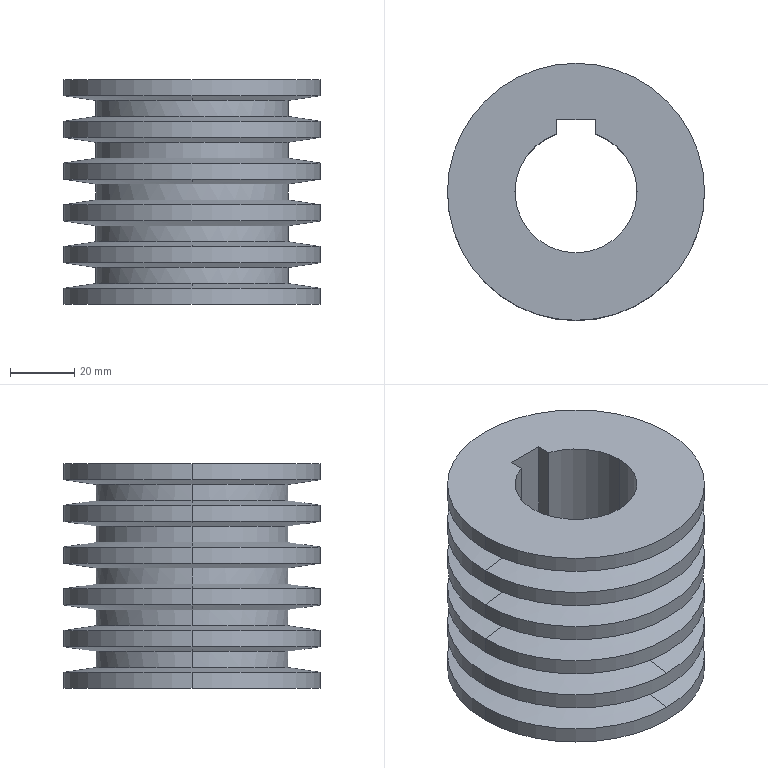Part | SolidWorks | 1 solid | 50 faces | box 80 x 80 x 70 mm | volume 197004 mm3 | cylinder 25 | cone 20 | plane 5 | commonest cylinder face diameters 80 x12 60 x10 38 x3
STEP:
#1=CARTESIAN_POINT('',(6.,18.028,-70.));
#2=VERTEX_POINT('',#1);
#3=CARTESIAN_POINT('',(6.,18.028,0.));
#4=VERTEX_POINT('',#3);
#5=CARTESIAN_POINT('',(6.,18.028,-70.));
#6=DIRECTION('',(0.,0.,1.));
#7=VECTOR('',#6,1000.);
#8=LINE('',#5,#7);
#9=EDGE_CURVE('',#2,#4,#8,.T.);
#10=ORIENTED_EDGE('',*,*,#9,.T.);
#11=CARTESIAN_POINT('',(6.,22.5,0.));
#12=VERTEX_POINT('',#11);
#13=CARTESIAN_POINT('',(6.,22.5,0.));
#14=DIRECTION('',(0.,-1.,0.));
#15=VECTOR('',#14,1000.);
#16=LINE('',#13,#15);
#17=EDGE_CURVE('',#12,#4,#16,.T.);
#18=ORIENTED_EDGE('',*,*,#17,.F.);
#19=CARTESIAN_POINT('',(6.,22.5,-70.));
#20=VERTEX_POINT('',#19);
#21=CARTESIAN_POINT('',(6.,22.5,0.));
#22=DIRECTION('',(0.,0.,-1.));
#23=VECTOR('',#22,1000.);
#24=LINE('',#21,#23);
#25=EDGE_CURVE('',#12,#20,#24,.T.);
#26=ORIENTED_EDGE('',*,*,#25,.T.);
#27=CARTESIAN_POINT('',(6.,18.028,-70.));
#28=DIRECTION('',(0.,1.,0.));
#29=VECTOR('',#28,1000.);
#30=LINE('',#27,#29);
#31=EDGE_CURVE('',#2,#20,#30,.T.);
#32=ORIENTED_EDGE('',*,*,#31,.F.);
#33=EDGE_LOOP('',(#10,#18,#26,#32));
#34=FACE_OUTER_BOUND('',#33,.T.);
#35=CARTESIAN_POINT('',(6.,22.5,-70.));
#36=DIRECTION('',(1.,0.,0.));
#37=DIRECTION('',(0.,1.,0.));
#38=AXIS2_PLACEMENT_3D('',#35,#36,#37);
#39=PLANE('',#38);
#40=ADVANCED_FACE('',(#34),#39,.F.);
#41=CARTESIAN_POINT('',(19.,0.,0.));
#42=VERTEX_POINT('',#41);
#43=CARTESIAN_POINT('',(0.,0.,0.));
#44=DIRECTION('',(0.,0.,1.));
#45=DIRECTION('',(1.,0.,0.));
#46=AXIS2_PLACEMENT_3D('',#43,#44,#45);
#47=CIRCLE('',#46,19.);
#48=EDGE_CURVE('',#42,#4,#47,.T.);
#49=ORIENTED_EDGE('',*,*,#48,.T.);
#50=ORIENTED_EDGE('',*,*,#9,.F.);
#51=CARTESIAN_POINT('',(19.,0.,-70.));
#52=VERTEX_POINT('',#51);
#53=CARTESIAN_POINT('',(0.,0.,-70.));
#54=DIRECTION('',(0.,0.,-1.));
#55=DIRECTION('',(0.3158,0.9488,0.));
#56=AXIS2_PLACEMENT_3D('',#53,#54,#55);
#57=CIRCLE('',#56,19.);
#58=EDGE_CURVE('',#2,#52,#57,.T.);
#59=ORIENTED_EDGE('',*,*,#58,.T.);
#60=CARTESIAN_POINT('',(19.,0.,-70.));
#61=DIRECTION('',(0.,0.,1.));
#62=VECTOR('',#61,1000.);
#63=LINE('',#60,#62);
#64=EDGE_CURVE('',#52,#42,#63,.T.);
#65=ORIENTED_EDGE('',*,*,#64,.T.);
#66=EDGE_LOOP('',(#49,#50,#59,#65));
#67=FACE_OUTER_BOUND('',#66,.T.);
#68=CARTESIAN_POINT('',(0.,0.,0.));
#69=DIRECTION('',(0.,0.,1.));
#70=DIRECTION('',(1.,0.,0.));
#71=AXIS2_PLACEMENT_3D('',#68,#69,#70);
#72=CYLINDRICAL_SURFACE('',#71,19.);
#73=ADVANCED_FACE('',(#67),#72,.F.);
#74=CARTESIAN_POINT('',(-6.,22.5,0.));
#75=VERTEX_POINT('',#74);
#76=CARTESIAN_POINT('',(-6.,22.5,-70.));
#77=VERTEX_POINT('',#76);
#78=CARTESIAN_POINT('',(-6.,22.5,0.));
#79=DIRECTION('',(0.,0.,-1.));
#80=VECTOR('',#79,1000.);
#81=LINE('',#78,#80);
#82=EDGE_CURVE('',#75,#77,#81,.T.);
#83=ORIENTED_EDGE('',*,*,#82,.F.);
#84=CARTESIAN_POINT('',(-6.,18.028,0.));
#85=VERTEX_POINT('',#84);
#86=CARTESIAN_POINT('',(-6.,18.028,0.));
#87=DIRECTION('',(0.,1.,0.));
#88=VECTOR('',#87,1000.);
#89=LINE('',#86,#88);
#90=EDGE_CURVE('',#85,#75,#89,.T.);
#91=ORIENTED_EDGE('',*,*,#90,.F.);
#92=CARTESIAN_POINT('',(-6.,18.028,-70.));
#93=VERTEX_POINT('',#92);
#94=CARTESIAN_POINT('',(-6.,18.028,0.));
#95=DIRECTION('',(0.,0.,-1.));
#96=VECTOR('',#95,1000.);
#97=LINE('',#94,#96);
#98=EDGE_CURVE('',#85,#93,#97,.T.);
#99=ORIENTED_EDGE('',*,*,#98,.T.);
#100=CARTESIAN_POINT('',(-6.,22.5,-70.));
#101=DIRECTION('',(0.,-1.,0.));
#102=VECTOR('',#101,1000.);
#103=LINE('',#100,#102);
#104=EDGE_CURVE('',#77,#93,#103,.T.);
#105=ORIENTED_EDGE('',*,*,#104,.F.);
#106=EDGE_LOOP('',(#83,#91,#99,#105));
#107=FACE_OUTER_BOUND('',#106,.T.);
#108=CARTESIAN_POINT('',(-6.,22.5,-70.));
#109=DIRECTION('',(-1.,0.,0.));
#110=DIRECTION('',(0.,0.,1.));
#111=AXIS2_PLACEMENT_3D('',#108,#109,#110);
#112=PLANE('',#111);
#113=ADVANCED_FACE('',(#107),#112,.F.);
#114=ORIENTED_EDGE('',*,*,#98,.F.);
#115=CARTESIAN_POINT('',(-19.,0.,0.));
#116=VERTEX_POINT('',#115);
#117=CARTESIAN_POINT('',(0.,0.,0.));
#118=DIRECTION('',(0.,0.,1.));
#119=DIRECTION('',(-0.3158,0.9488,0.));
#120=AXIS2_PLACEMENT_3D('',#117,#118,#119);
#121=CIRCLE('',#120,19.);
#122=EDGE_CURVE('',#85,#116,#121,.T.);
#123=ORIENTED_EDGE('',*,*,#122,.T.);
#124=CARTESIAN_POINT('',(-19.,0.,-70.));
#125=VERTEX_POINT('',#124);
#126=CARTESIAN_POINT('',(-19.,0.,-70.));
#127=DIRECTION('',(0.,0.,1.));
#128=VECTOR('',#127,1000.);
#129=LINE('',#126,#128);
#130=EDGE_CURVE('',#125,#116,#129,.T.);
#131=ORIENTED_EDGE('',*,*,#130,.F.);
#132=CARTESIAN_POINT('',(0.,0.,-70.));
#133=DIRECTION('',(0.,0.,-1.));
#134=DIRECTION('',(-1.,0.,0.));
#135=AXIS2_PLACEMENT_3D('',#132,#133,#134);
#136=CIRCLE('',#135,19.);
#137=EDGE_CURVE('',#125,#93,#136,.T.);
#138=ORIENTED_EDGE('',*,*,#137,.T.);
#139=EDGE_LOOP('',(#114,#123,#131,#138));
#140=FACE_OUTER_BOUND('',#139,.T.);
#141=CARTESIAN_POINT('',(0.,0.,0.));
#142=DIRECTION('',(0.,0.,1.));
#143=DIRECTION('',(1.,0.,0.));
#144=AXIS2_PLACEMENT_3D('',#141,#142,#143);
#145=CYLINDRICAL_SURFACE('',#144,19.);
#146=ADVANCED_FACE('',(#140),#145,.F.);
#147=CARTESIAN_POINT('',(0.,0.,0.));
#148=DIRECTION('',(0.,0.,1.));
#149=DIRECTION('',(-1.,0.,0.));
#150=AXIS2_PLACEMENT_3D('',#147,#148,#149);
#151=CIRCLE('',#150,19.);
#152=EDGE_CURVE('',#116,#42,#151,.T.);
#153=ORIENTED_EDGE('',*,*,#152,.T.);
#154=ORIENTED_EDGE('',*,*,#64,.F.);
#155=CARTESIAN_POINT('',(0.,0.,-70.));
#156=DIRECTION('',(0.,0.,-1.));
#157=DIRECTION('',(1.,0.,0.));
#158=AXIS2_PLACEMENT_3D('',#155,#156,#157);
#159=CIRCLE('',#158,19.);
#160=EDGE_CURVE('',#52,#125,#159,.T.);
#161=ORIENTED_EDGE('',*,*,#160,.T.);
#162=ORIENTED_EDGE('',*,*,#130,.T.);
#163=EDGE_LOOP('',(#153,#154,#161,#162));
#164=FACE_OUTER_BOUND('',#163,.T.);
#165=CARTESIAN_POINT('',(0.,0.,0.));
#166=DIRECTION('',(0.,0.,1.));
#167=DIRECTION('',(1.,0.,0.));
#168=AXIS2_PLACEMENT_3D('',#165,#166,#167);
#169=CYLINDRICAL_SURFACE('',#168,19.);
#170=ADVANCED_FACE('',(#164),#169,.F.);
#171=CARTESIAN_POINT('',(-40.,0.,-52.));
#172=VERTEX_POINT('',#171);
#173=CARTESIAN_POINT('',(0.,40.,-52.));
#174=VERTEX_POINT('',#173);
#175=CARTESIAN_POINT('',(0.,0.,-52.));
#176=DIRECTION('',(0.,0.,-1.));
#177=DIRECTION('',(-1.,0.,0.));
#178=AXIS2_PLACEMENT_3D('',#175,#176,#177);
#179=CIRCLE('',#178,40.);
#180=EDGE_CURVE('',#172,#174,#179,.T.);
#181=ORIENTED_EDGE('',*,*,#180,.T.);
#182=CARTESIAN_POINT('',(40.,0.,-52.));
#183=VERTEX_POINT('',#182);
#184=CARTESIAN_POINT('',(0.,0.,-52.));
#185=DIRECTION('',(0.,0.,-1.));
#186=DIRECTION('',(0.,1.,0.));
#187=AXIS2_PLACEMENT_3D('',#184,#185,#186);
#188=CIRCLE('',#187,40.);
#189=EDGE_CURVE('',#174,#183,#188,.T.);
#190=ORIENTED_EDGE('',*,*,#189,.T.);
#191=CARTESIAN_POINT('',(40.,0.,-57.));
#192=VERTEX_POINT('',#191);
#193=CARTESIAN_POINT('',(40.,0.,-57.));
#194=DIRECTION('',(0.,0.,1.));
#195=VECTOR('',#194,1000.);
#196=LINE('',#193,#195);
#197=EDGE_CURVE('',#192,#183,#196,.T.);
#198=ORIENTED_EDGE('',*,*,#197,.F.);
#199=CARTESIAN_POINT('',(-40.,0.,-57.));
#200=VERTEX_POINT('',#199);
#201=CARTESIAN_POINT('',(0.,0.,-57.));
#202=DIRECTION('',(0.,0.,1.));
#203=DIRECTION('',(1.,0.,0.));
#204=AXIS2_PLACEMENT_3D('',#201,#202,#203);
#205=CIRCLE('',#204,40.);
#206=EDGE_CURVE('',#192,#200,#205,.T.);
#207=ORIENTED_EDGE('',*,*,#206,.T.);
#208=CARTESIAN_POINT('',(-40.,0.,-57.));
#209=DIRECTION('',(0.,0.,1.));
#210=VECTOR('',#209,1000.);
#211=LINE('',#208,#210);
#212=EDGE_CURVE('',#200,#172,#211,.T.);
#213=ORIENTED_EDGE('',*,*,#212,.T.);
#214=EDGE_LOOP('',(#181,#190,#198,#207,#213));
#215=FACE_OUTER_BOUND('',#214,.T.);
#216=CARTESIAN_POINT('',(0.,0.,0.));
#217=DIRECTION('',(0.,0.,1.));
#218=DIRECTION('',(1.,0.,0.));
#219=AXIS2_PLACEMENT_3D('',#216,#217,#218);
#220=CYLINDRICAL_SURFACE('',#219,40.);
#221=ADVANCED_FACE('',(#215),#220,.T.);
#222=ORIENTED_EDGE('',*,*,#197,.T.);
#223=CARTESIAN_POINT('',(0.,-40.,-52.));
#224=VERTEX_POINT('',#223);
#225=CARTESIAN_POINT('',(0.,0.,-52.));
#226=DIRECTION('',(0.,0.,-1.));
#227=DIRECTION('',(1.,0.,0.));
#228=AXIS2_PLACEMENT_3D('',#225,#226,#227);
#229=CIRCLE('',#228,40.);
#230=EDGE_CURVE('',#183,#224,#229,.T.);
#231=ORIENTED_EDGE('',*,*,#230,.T.);
#232=CARTESIAN_POINT('',(0.,0.,-52.));
#233=DIRECTION('',(0.,0.,-1.));
#234=DIRECTION('',(0.,-1.,0.));
#235=AXIS2_PLACEMENT_3D('',#232,#233,#234);
#236=CIRCLE('',#235,40.);
#237=EDGE_CURVE('',#224,#172,#236,.T.);
#238=ORIENTED_EDGE('',*,*,#237,.T.);
#239=ORIENTED_EDGE('',*,*,#212,.F.);
#240=CARTESIAN_POINT('',(0.,0.,-57.));
#241=DIRECTION('',(0.,0.,1.));
#242=DIRECTION('',(-1.,0.,0.));
#243=AXIS2_PLACEMENT_3D('',#240,#241,#242);
#244=CIRCLE('',#243,40.);
#245=EDGE_CURVE('',#200,#192,#244,.T.);
#246=ORIENTED_EDGE('',*,*,#245,.T.);
#247=EDGE_LOOP('',(#222,#231,#238,#239,#246));
#248=FACE_OUTER_BOUND('',#247,.T.);
#249=CARTESIAN_POINT('',(0.,0.,0.));
#250=DIRECTION('',(0.,0.,1.));
#251=DIRECTION('',(1.,0.,0.));
#252=AXIS2_PLACEMENT_3D('',#249,#250,#251);
#253=CYLINDRICAL_SURFACE('',#252,40.);
#254=ADVANCED_FACE('',(#248),#253,.T.);
#255=CARTESIAN_POINT('',(30.,0.,-58.5));
#256=VERTEX_POINT('',#255);
#257=CARTESIAN_POINT('',(30.,0.,-58.5));
#258=DIRECTION('',(0.9889,0.,0.1483));
#259=VECTOR('',#258,1000.);
#260=LINE('',#257,#259);
#261=EDGE_CURVE('',#256,#192,#260,.T.);
#262=ORIENTED_EDGE('',*,*,#261,.T.);
#263=ORIENTED_EDGE('',*,*,#245,.F.);
#264=CARTESIAN_POINT('',(-30.,0.,-58.5));
#265=VERTEX_POINT('',#264);
#266=CARTESIAN_POINT('',(-30.,0.,-58.5));
#267=DIRECTION('',(-0.9889,0.,0.1483));
#268=VECTOR('',#267,1000.);
#269=LINE('',#266,#268);
#270=EDGE_CURVE('',#265,#200,#269,.T.);
#271=ORIENTED_EDGE('',*,*,#270,.F.);
#272=CARTESIAN_POINT('',(0.,0.,-58.5));
#273=DIRECTION('',(0.,0.,-1.));
#274=DIRECTION('',(1.,0.,0.));
#275=AXIS2_PLACEMENT_3D('',#272,#273,#274);
#276=CIRCLE('',#275,30.);
#277=EDGE_CURVE('',#256,#265,#276,.T.);
#278=ORIENTED_EDGE('',*,*,#277,.F.);
#279=EDGE_LOOP('',(#262,#263,#271,#278));
#280=FACE_OUTER_BOUND('',#279,.T.);
#281=CARTESIAN_POINT('',(0.,0.,-58.53));
#282=DIRECTION('',(0.,0.,1.));
#283=DIRECTION('',(1.,0.,0.));
#284=AXIS2_PLACEMENT_3D('',#281,#282,#283);
#285=CONICAL_SURFACE('',#284,29.8,1.422);
#286=ADVANCED_FACE('',(#280),#285,.T.);
#287=ORIENTED_EDGE('',*,*,#206,.F.);
#288=ORIENTED_EDGE('',*,*,#261,.F.);
#289=CARTESIAN_POINT('',(0.,0.,-58.5));
#290=DIRECTION('',(0.,0.,-1.));
#291=DIRECTION('',(-1.,0.,0.));
#292=AXIS2_PLACEMENT_3D('',#289,#290,#291);
#293=CIRCLE('',#292,30.);
#294=EDGE_CURVE('',#265,#256,#293,.T.);
#295=ORIENTED_EDGE('',*,*,#294,.F.);
#296=ORIENTED_EDGE('',*,*,#270,.T.);
#297=EDGE_LOOP('',(#287,#288,#295,#296));
#298=FACE_OUTER_BOUND('',#297,.T.);
#299=CARTESIAN_POINT('',(0.,0.,-58.53));
#300=DIRECTION('',(0.,0.,1.));
#301=DIRECTION('',(1.,0.,0.));
#302=AXIS2_PLACEMENT_3D('',#299,#300,#301);
#303=CONICAL_SURFACE('',#302,29.8,1.422);
#304=ADVANCED_FACE('',(#298),#303,.T.);
#305=CARTESIAN_POINT('',(40.,0.,-65.));
#306=VERTEX_POINT('',#305);
#307=CARTESIAN_POINT('',(0.,-40.,-65.));
#308=VERTEX_POINT('',#307);
#309=CARTESIAN_POINT('',(0.,0.,-65.));
#310=DIRECTION('',(0.,0.,-1.));
#311=DIRECTION('',(1.,0.,0.));
#312=AXIS2_PLACEMENT_3D('',#309,#310,#311);
#313=CIRCLE('',#312,40.);
#314=EDGE_CURVE('',#306,#308,#313,.T.);
#315=ORIENTED_EDGE('',*,*,#314,.F.);
#316=CARTESIAN_POINT('',(0.,40.,-65.));
#317=VERTEX_POINT('',#316);
#318=CARTESIAN_POINT('',(0.,0.,-65.));
#319=DIRECTION('',(0.,0.,-1.));
#320=DIRECTION('',(0.,1.,0.));
#321=AXIS2_PLACEMENT_3D('',#318,#319,#320);
#322=CIRCLE('',#321,40.);
#323=EDGE_CURVE('',#317,#306,#322,.T.);
#324=ORIENTED_EDGE('',*,*,#323,.F.);
#325=CARTESIAN_POINT('',(0.,30.,-63.5));
#326=VERTEX_POINT('',#325);
#327=CARTESIAN_POINT('',(0.,30.,-63.5));
#328=DIRECTION('',(0.,0.9889,-0.1483));
#329=VECTOR('',#328,1000.);
#330=LINE('',#327,#329);
#331=EDGE_CURVE('',#326,#317,#330,.T.);
#332=ORIENTED_EDGE('',*,*,#331,.F.);
#333=CARTESIAN_POINT('',(30.,0.,-63.5));
#334=VERTEX_POINT('',#333);
#335=CARTESIAN_POINT('',(0.,0.,-63.5));
#336=DIRECTION('',(0.,0.,1.));
#337=DIRECTION('',(1.,0.,0.));
#338=AXIS2_PLACEMENT_3D('',#335,#336,#337);
#339=CIRCLE('',#338,30.);
#340=EDGE_CURVE('',#334,#326,#339,.T.);
#341=ORIENTED_EDGE('',*,*,#340,.F.);
#342=CARTESIAN_POINT('',(0.,-30.,-63.5));
#343=VERTEX_POINT('',#342);
#344=CARTESIAN_POINT('',(0.,0.,-63.5));
#345=DIRECTION('',(0.,0.,1.));
#346=DIRECTION('',(0.,-1.,0.));
#347=AXIS2_PLACEMENT_3D('',#344,#345,#346);
#348=CIRCLE('',#347,30.);
#349=EDGE_CURVE('',#343,#334,#348,.T.);
#350=ORIENTED_EDGE('',*,*,#349,.F.);
#351=CARTESIAN_POINT('',(0.,-30.,-63.5));
#352=DIRECTION('',(0.,-0.9889,-0.1483));
#353=VECTOR('',#352,1000.);
#354=LINE('',#351,#353);
#355=EDGE_CURVE('',#343,#308,#354,.T.);
#356=ORIENTED_EDGE('',*,*,#355,.T.);
#357=EDGE_LOOP('',(#315,#324,#332,#341,#350,#356));
#358=FACE_OUTER_BOUND('',#357,.T.);
#359=CARTESIAN_POINT('',(0.,0.,-63.47));
#360=DIRECTION('',(0.,0.,-1.));
#361=DIRECTION('',(0.,1.,0.));
#362=AXIS2_PLACEMENT_3D('',#359,#360,#361);
#363=CONICAL_SURFACE('',#362,29.8,1.422);
#364=ADVANCED_FACE('',(#358),#363,.T.);
#365=ORIENTED_EDGE('',*,*,#294,.T.);
#366=CARTESIAN_POINT('',(30.,0.,-63.5));
#367=DIRECTION('',(0.,0.,1.));
#368=VECTOR('',#367,1000.);
#369=LINE('',#366,#368);
#370=EDGE_CURVE('',#334,#256,#369,.T.);
#371=ORIENTED_EDGE('',*,*,#370,.F.);
#372=ORIENTED_EDGE('',*,*,#340,.T.);
#373=CARTESIAN_POINT('',(-30.,0.,-63.5));
#374=VERTEX_POINT('',#373);
#375=CARTESIAN_POINT('',(0.,0.,-63.5));
#376=DIRECTION('',(0.,0.,1.));
#377=DIRECTION('',(0.,1.,0.));
#378=AXIS2_PLACEMENT_3D('',#375,#376,#377);
#379=CIRCLE('',#378,30.);
#380=EDGE_CURVE('',#326,#374,#379,.T.);
#381=ORIENTED_EDGE('',*,*,#380,.T.);
#382=CARTESIAN_POINT('',(-30.,0.,-63.5));
#383=DIRECTION('',(0.,0.,1.));
#384=VECTOR('',#383,1000.);
#385=LINE('',#382,#384);
#386=EDGE_CURVE('',#374,#265,#385,.T.);
#387=ORIENTED_EDGE('',*,*,#386,.T.);
#388=EDGE_LOOP('',(#365,#371,#372,#381,#387));
#389=FACE_OUTER_BOUND('',#388,.T.);
#390=CARTESIAN_POINT('',(0.,0.,0.));
#391=DIRECTION('',(0.,0.,1.));
#392=DIRECTION('',(1.,0.,0.));
#393=AXIS2_PLACEMENT_3D('',#390,#391,#392);
#394=CYLINDRICAL_SURFACE('',#393,30.);
#395=ADVANCED_FACE('',(#389),#394,.T.);
#396=ORIENTED_EDGE('',*,*,#349,.T.);
#397=ORIENTED_EDGE('',*,*,#370,.T.);
#398=ORIENTED_EDGE('',*,*,#277,.T.);
#399=ORIENTED_EDGE('',*,*,#386,.F.);
#400=CARTESIAN_POINT('',(0.,0.,-63.5));
#401=DIRECTION('',(0.,0.,1.));
#402=DIRECTION('',(-1.,0.,0.));
#403=AXIS2_PLACEMENT_3D('',#400,#401,#402);
#404=CIRCLE('',#403,30.);
#405=EDGE_CURVE('',#374,#343,#404,.T.);
#406=ORIENTED_EDGE('',*,*,#405,.T.);
#407=EDGE_LOOP('',(#396,#397,#398,#399,#406));
#408=FACE_OUTER_BOUND('',#407,.T.);
#409=CARTESIAN_POINT('',(0.,0.,0.));
#410=DIRECTION('',(0.,0.,1.));
#411=DIRECTION('',(1.,0.,0.));
#412=AXIS2_PLACEMENT_3D('',#409,#410,#411);
#413=CYLINDRICAL_SURFACE('',#412,30.);
#414=ADVANCED_FACE('',(#408),#413,.T.);
#415=ORIENTED_EDGE('',*,*,#380,.F.);
#416=ORIENTED_EDGE('',*,*,#331,.T.);
#417=CARTESIAN_POINT('',(-40.,0.,-65.));
#418=VERTEX_POINT('',#417);
#419=CARTESIAN_POINT('',(0.,0.,-65.));
#420=DIRECTION('',(0.,0.,-1.));
#421=DIRECTION('',(-1.,0.,0.));
#422=AXIS2_PLACEMENT_3D('',#419,#420,#421);
#423=CIRCLE('',#422,40.);
#424=EDGE_CURVE('',#418,#317,#423,.T.);
#425=ORIENTED_EDGE('',*,*,#424,.F.);
#426=CARTESIAN_POINT('',(0.,0.,-65.));
#427=DIRECTION('',(0.,0.,-1.));
#428=DIRECTION('',(0.,-1.,0.));
#429=AXIS2_PLACEMENT_3D('',#426,#427,#428);
#430=CIRCLE('',#429,40.);
#431=EDGE_CURVE('',#308,#418,#430,.T.);
#432=ORIENTED_EDGE('',*,*,#431,.F.);
#433=ORIENTED_EDGE('',*,*,#355,.F.);
#434=ORIENTED_EDGE('',*,*,#405,.F.);
#435=EDGE_LOOP('',(#415,#416,#425,#432,#433,#434));
#436=FACE_OUTER_BOUND('',#435,.T.);
#437=CARTESIAN_POINT('',(0.,0.,-63.47));
#438=DIRECTION('',(0.,0.,-1.));
#439=DIRECTION('',(0.,1.,0.));
#440=AXIS2_PLACEMENT_3D('',#437,#438,#439);
#441=CONICAL_SURFACE('',#440,29.8,1.422);
#442=ADVANCED_FACE('',(#436),#441,.T.);
#443=CARTESIAN_POINT('',(40.,0.,-70.));
#444=VERTEX_POINT('',#443);
#445=CARTESIAN_POINT('',(40.,0.,-70.));
#446=DIRECTION('',(0.,0.,1.));
#447=VECTOR('',#446,1000.);
#448=LINE('',#445,#447);
#449=EDGE_CURVE('',#444,#306,#448,.T.);
#450=ORIENTED_EDGE('',*,*,#449,.T.);
#451=ORIENTED_EDGE('',*,*,#314,.T.);
#452=ORIENTED_EDGE('',*,*,#431,.T.);
#453=CARTESIAN_POINT('',(-40.,0.,-70.));
#454=VERTEX_POINT('',#453);
#455=CARTESIAN_POINT('',(-40.,0.,-70.));
#456=DIRECTION('',(0.,0.,1.));
#457=VECTOR('',#456,1000.);
#458=LINE('',#455,#457);
#459=EDGE_CURVE('',#454,#418,#458,.T.);
#460=ORIENTED_EDGE('',*,*,#459,.F.);
#461=CARTESIAN_POINT('',(0.,0.,-70.));
#462=DIRECTION('',(0.,0.,1.));
#463=DIRECTION('',(-1.,0.,0.));
#464=AXIS2_PLACEMENT_3D('',#461,#462,#463);
#465=CIRCLE('',#464,40.);
#466=EDGE_CURVE('',#454,#444,#465,.T.);
#467=ORIENTED_EDGE('',*,*,#466,.T.);
#468=EDGE_LOOP('',(#450,#451,#452,#460,#467));
#469=FACE_OUTER_BOUND('',#468,.T.);
#470=CARTESIAN_POINT('',(0.,0.,0.));
#471=DIRECTION('',(0.,0.,1.));
#472=DIRECTION('',(1.,0.,0.));
#473=AXIS2_PLACEMENT_3D('',#470,#471,#472);
#474=CYLINDRICAL_SURFACE('',#473,40.);
#475=ADVANCED_FACE('',(#469),#474,.T.);
#476=ORIENTED_EDGE('',*,*,#424,.T.);
#477=ORIENTED_EDGE('',*,*,#323,.T.);
#478=ORIENTED_EDGE('',*,*,#449,.F.);
#479=CARTESIAN_POINT('',(0.,0.,-70.));
#480=DIRECTION('',(0.,0.,1.));
#481=DIRECTION('',(1.,0.,0.));
#482=AXIS2_PLACEMENT_3D('',#479,#480,#481);
#483=CIRCLE('',#482,40.);
#484=EDGE_CURVE('',#444,#454,#483,.T.);
#485=ORIENTED_EDGE('',*,*,#484,.T.);
#486=ORIENTED_EDGE('',*,*,#459,.T.);
#487=EDGE_LOOP('',(#476,#477,#478,#485,#486));
#488=FACE_OUTER_BOUND('',#487,.T.);
#489=CARTESIAN_POINT('',(0.,0.,0.));
#490=DIRECTION('',(0.,0.,1.));
#491=DIRECTION('',(1.,0.,0.));
#492=AXIS2_PLACEMENT_3D('',#489,#490,#491);
#493=CYLINDRICAL_SURFACE('',#492,40.);
#494=ADVANCED_FACE('',(#488),#493,.T.);
#495=ORIENTED_EDGE('',*,*,#58,.F.);
#496=ORIENTED_EDGE('',*,*,#31,.T.);
#497=CARTESIAN_POINT('',(6.,22.5,-70.));
#498=DIRECTION('',(-1.,0.,0.));
#499=VECTOR('',#498,1000.);
#500=LINE('',#497,#499);
#501=EDGE_CURVE('',#20,#77,#500,.T.);
#502=ORIENTED_EDGE('',*,*,#501,.T.);
#503=ORIENTED_EDGE('',*,*,#104,.T.);
#504=ORIENTED_EDGE('',*,*,#137,.F.);
#505=ORIENTED_EDGE('',*,*,#160,.F.);
#506=EDGE_LOOP('',(#495,#496,#502,#503,#504,#505));
#507=FACE_BOUND('',#506,.T.);
#508=ORIENTED_EDGE('',*,*,#466,.F.);
#509=ORIENTED_EDGE('',*,*,#484,.F.);
#510=EDGE_LOOP('',(#508,#509));
#511=FACE_OUTER_BOUND('',#510,.T.);
#512=CARTESIAN_POINT('',(0.,-40.,-70.));
#513=DIRECTION('',(0.,0.,-1.));
#514=DIRECTION('',(0.,-1.,0.));
#515=AXIS2_PLACEMENT_3D('',#512,#513,#514);
#516=PLANE('',#515);
#517=ADVANCED_FACE('',(#507,#511),#516,.T.);
#518=ORIENTED_EDGE('',*,*,#25,.F.);
#519=CARTESIAN_POINT('',(-6.,22.5,0.));
#520=DIRECTION('',(1.,0.,0.));
#521=VECTOR('',#520,1000.);
#522=LINE('',#519,#521);
#523=EDGE_CURVE('',#75,#12,#522,.T.);
#524=ORIENTED_EDGE('',*,*,#523,.F.);
#525=ORIENTED_EDGE('',*,*,#82,.T.);
#526=ORIENTED_EDGE('',*,*,#501,.F.);
#527=EDGE_LOOP('',(#518,#524,#525,#526));
#528=FACE_OUTER_BOUND('',#527,.T.);
#529=CARTESIAN_POINT('',(0.,22.5,-70.));
#530=DIRECTION('',(0.,1.,0.));
#531=DIRECTION('',(1.,0.,0.));
#532=AXIS2_PLACEMENT_3D('',#529,#530,#531);
#533=PLANE('',#532);
#534=ADVANCED_FACE('',(#528),#533,.F.);
#535=ORIENTED_EDGE('',*,*,#17,.T.);
#536=ORIENTED_EDGE('',*,*,#48,.F.);
#537=ORIENTED_EDGE('',*,*,#152,.F.);
#538=ORIENTED_EDGE('',*,*,#122,.F.);
#539=ORIENTED_EDGE('',*,*,#90,.T.);
#540=ORIENTED_EDGE('',*,*,#523,.T.);
#541=EDGE_LOOP('',(#535,#536,#537,#538,#539,#540));
#542=FACE_BOUND('',#541,.T.);
#543=CARTESIAN_POINT('',(-40.,0.,0.));
#544=VERTEX_POINT('',#543);
#545=CARTESIAN_POINT('',(40.,0.,0.));
#546=VERTEX_POINT('',#545);
#547=CARTESIAN_POINT('',(0.,0.,0.));
#548=DIRECTION('',(0.,0.,-1.));
#549=DIRECTION('',(-1.,0.,0.));
#550=AXIS2_PLACEMENT_3D('',#547,#548,#549);
#551=CIRCLE('',#550,40.);
#552=EDGE_CURVE('',#544,#546,#551,.T.);
#553=ORIENTED_EDGE('',*,*,#552,.F.);
#554=CARTESIAN_POINT('',(0.,0.,0.));
#555=DIRECTION('',(0.,0.,-1.));
#556=DIRECTION('',(1.,0.,0.));
#557=AXIS2_PLACEMENT_3D('',#554,#555,#556);
#558=CIRCLE('',#557,40.);
#559=EDGE_CURVE('',#546,#544,#558,.T.);
#560=ORIENTED_EDGE('',*,*,#559,.F.);
#561=EDGE_LOOP('',(#553,#560));
#562=FACE_OUTER_BOUND('',#561,.T.);
#563=CARTESIAN_POINT('',(0.,-19.,0.));
#564=DIRECTION('',(0.,0.,1.));
#565=DIRECTION('',(1.,0.,0.));
#566=AXIS2_PLACEMENT_3D('',#563,#564,#565);
#567=PLANE('',#566);
#568=ADVANCED_FACE('',(#542,#562),#567,.T.);
#569=CARTESIAN_POINT('',(0.,-40.,-5.));
#570=VERTEX_POINT('',#569);
#571=CARTESIAN_POINT('',(40.,0.,-5.));
#572=VERTEX_POINT('',#571);
#573=CARTESIAN_POINT('',(0.,0.,-5.));
#574=DIRECTION('',(0.,0.,1.));
#575=DIRECTION('',(0.,-1.,0.));
#576=AXIS2_PLACEMENT_3D('',#573,#574,#575);
#577=CIRCLE('',#576,40.);
#578=EDGE_CURVE('',#570,#572,#577,.T.);
#579=ORIENTED_EDGE('',*,*,#578,.T.);
#580=CARTESIAN_POINT('',(40.,0.,-5.));
#581=DIRECTION('',(0.,0.,1.));
#582=VECTOR('',#581,1000.);
#583=LINE('',#580,#582);
#584=EDGE_CURVE('',#572,#546,#583,.T.);
#585=ORIENTED_EDGE('',*,*,#584,.T.);
#586=ORIENTED_EDGE('',*,*,#559,.T.);
#587=CARTESIAN_POINT('',(-40.,0.,-5.));
#588=VERTEX_POINT('',#587);
#589=CARTESIAN_POINT('',(-40.,0.,-5.));
#590=DIRECTION('',(0.,0.,1.));
#591=VECTOR('',#590,1000.);
#592=LINE('',#589,#591);
#593=EDGE_CURVE('',#588,#544,#592,.T.);
#594=ORIENTED_EDGE('',*,*,#593,.F.);
#595=CARTESIAN_POINT('',(0.,0.,-5.));
#596=DIRECTION('',(0.,0.,1.));
#597=DIRECTION('',(-1.,0.,0.));
#598=AXIS2_PLACEMENT_3D('',#595,#596,#597);
#599=CIRCLE('',#598,40.);
#600=EDGE_CURVE('',#588,#570,#599,.T.);
#601=ORIENTED_EDGE('',*,*,#600,.T.);
#602=EDGE_LOOP('',(#579,#585,#586,#594,#601));
#603=FACE_OUTER_BOUND('',#602,.T.);
#604=CARTESIAN_POINT('',(0.,0.,0.));
#605=DIRECTION('',(0.,0.,1.));
#606=DIRECTION('',(1.,0.,0.));
#607=AXIS2_PLACEMENT_3D('',#604,#605,#606);
#608=CYLINDRICAL_SURFACE('',#607,40.);
#609=ADVANCED_FACE('',(#603),#608,.T.);
#610=ORIENTED_EDGE('',*,*,#552,.T.);
#611=ORIENTED_EDGE('',*,*,#584,.F.);
#612=CARTESIAN_POINT('',(0.,40.,-5.));
#613=VERTEX_POINT('',#612);
#614=CARTESIAN_POINT('',(0.,0.,-5.));
#615=DIRECTION('',(0.,0.,1.));
#616=DIRECTION('',(1.,0.,0.));
#617=AXIS2_PLACEMENT_3D('',#614,#615,#616);
#618=CIRCLE('',#617,40.);
#619=EDGE_CURVE('',#572,#613,#618,.T.);
#620=ORIENTED_EDGE('',*,*,#619,.T.);
#621=CARTESIAN_POINT('',(0.,0.,-5.));
#622=DIRECTION('',(0.,0.,1.));
#623=DIRECTION('',(0.,1.,0.));
#624=AXIS2_PLACEMENT_3D('',#621,#622,#623);
#625=CIRCLE('',#624,40.);
#626=EDGE_CURVE('',#613,#588,#625,.T.);
#627=ORIENTED_EDGE('',*,*,#626,.T.);
#628=ORIENTED_EDGE('',*,*,#593,.T.);
#629=EDGE_LOOP('',(#610,#611,#620,#627,#628));
#630=FACE_OUTER_BOUND('',#629,.T.);
#631=CARTESIAN_POINT('',(0.,0.,0.));
#632=DIRECTION('',(0.,0.,1.));
#633=DIRECTION('',(1.,0.,0.));
#634=AXIS2_PLACEMENT_3D('',#631,#632,#633);
#635=CYLINDRICAL_SURFACE('',#634,40.);
#636=ADVANCED_FACE('',(#630),#635,.T.);
#637=CARTESIAN_POINT('',(0.,-30.,-6.5));
#638=VERTEX_POINT('',#637);
#639=CARTESIAN_POINT('',(-30.,0.,-6.5));
#640=VERTEX_POINT('',#639);
#641=CARTESIAN_POINT('',(0.,0.,-6.5));
#642=DIRECTION('',(0.,0.,-1.));
#643=DIRECTION('',(0.,-1.,0.));
#644=AXIS2_PLACEMENT_3D('',#641,#642,#643);
#645=CIRCLE('',#644,30.);
#646=EDGE_CURVE('',#638,#640,#645,.T.);
#647=ORIENTED_EDGE('',*,*,#646,.F.);
#648=CARTESIAN_POINT('',(0.,-30.,-6.5));
#649=DIRECTION('',(0.,-0.9889,0.1483));
#650=VECTOR('',#649,1000.);
#651=LINE('',#648,#650);
#652=EDGE_CURVE('',#638,#570,#651,.T.);
#653=ORIENTED_EDGE('',*,*,#652,.T.);
#654=ORIENTED_EDGE('',*,*,#600,.F.);
#655=ORIENTED_EDGE('',*,*,#626,.F.);
#656=CARTESIAN_POINT('',(0.,30.,-6.5));
#657=VERTEX_POINT('',#656);
#658=CARTESIAN_POINT('',(0.,30.,-6.5));
#659=DIRECTION('',(0.,0.9889,0.1483));
#660=VECTOR('',#659,1000.);
#661=LINE('',#658,#660);
#662=EDGE_CURVE('',#657,#613,#661,.T.);
#663=ORIENTED_EDGE('',*,*,#662,.F.);
#664=CARTESIAN_POINT('',(0.,0.,-6.5));
#665=DIRECTION('',(0.,0.,-1.));
#666=DIRECTION('',(-1.,0.,0.));
#667=AXIS2_PLACEMENT_3D('',#664,#665,#666);
#668=CIRCLE('',#667,30.);
#669=EDGE_CURVE('',#640,#657,#668,.T.);
#670=ORIENTED_EDGE('',*,*,#669,.F.);
#671=EDGE_LOOP('',(#647,#653,#654,#655,#663,#670));
#672=FACE_OUTER_BOUND('',#671,.T.);
#673=CARTESIAN_POINT('',(0.,0.,-6.53));
#674=DIRECTION('',(0.,0.,1.));
#675=DIRECTION('',(0.,-1.,0.));
#676=AXIS2_PLACEMENT_3D('',#673,#674,#675);
#677=CONICAL_SURFACE('',#676,29.8,1.422);
#678=ADVANCED_FACE('',(#672),#677,.T.);
#679=ORIENTED_EDGE('',*,*,#619,.F.);
#680=ORIENTED_EDGE('',*,*,#578,.F.);
#681=ORIENTED_EDGE('',*,*,#652,.F.);
#682=CARTESIAN_POINT('',(30.,0.,-6.5));
#683=VERTEX_POINT('',#682);
#684=CARTESIAN_POINT('',(0.,0.,-6.5));
#685=DIRECTION('',(0.,0.,-1.));
#686=DIRECTION('',(1.,0.,0.));
#687=AXIS2_PLACEMENT_3D('',#684,#685,#686);
#688=CIRCLE('',#687,30.);
#689=EDGE_CURVE('',#683,#638,#688,.T.);
#690=ORIENTED_EDGE('',*,*,#689,.F.);
#691=CARTESIAN_POINT('',(0.,0.,-6.5));
#692=DIRECTION('',(0.,0.,-1.));
#693=DIRECTION('',(0.,1.,0.));
#694=AXIS2_PLACEMENT_3D('',#691,#692,#693);
#695=CIRCLE('',#694,30.);
#696=EDGE_CURVE('',#657,#683,#695,.T.);
#697=ORIENTED_EDGE('',*,*,#696,.F.);
#698=ORIENTED_EDGE('',*,*,#662,.T.);
#699=EDGE_LOOP('',(#679,#680,#681,#690,#697,#698));
#700=FACE_OUTER_BOUND('',#699,.T.);
#701=CARTESIAN_POINT('',(0.,0.,-6.53));
#702=DIRECTION('',(0.,0.,1.));
#703=DIRECTION('',(0.,-1.,0.));
#704=AXIS2_PLACEMENT_3D('',#701,#702,#703);
#705=CONICAL_SURFACE('',#704,29.8,1.422);
#706=ADVANCED_FACE('',(#700),#705,.T.);
#707=ORIENTED_EDGE('',*,*,#669,.T.);
#708=ORIENTED_EDGE('',*,*,#696,.T.);
#709=CARTESIAN_POINT('',(30.,0.,-11.5));
#710=VERTEX_POINT('',#709);
#711=CARTESIAN_POINT('',(30.,0.,-11.5));
#712=DIRECTION('',(0.,0.,1.));
#713=VECTOR('',#712,1000.);
#714=LINE('',#711,#713);
#715=EDGE_CURVE('',#710,#683,#714,.T.);
#716=ORIENTED_EDGE('',*,*,#715,.F.);
#717=CARTESIAN_POINT('',(-30.,0.,-11.5));
#718=VERTEX_POINT('',#717);
#719=CARTESIAN_POINT('',(0.,0.,-11.5));
#720=DIRECTION('',(0.,0.,1.));
#721=DIRECTION('',(1.,0.,0.));
#722=AXIS2_PLACEMENT_3D('',#719,#720,#721);
#723=CIRCLE('',#722,30.);
#724=EDGE_CURVE('',#710,#718,#723,.T.);
#725=ORIENTED_EDGE('',*,*,#724,.T.);
#726=CARTESIAN_POINT('',(-30.,0.,-11.5));
#727=DIRECTION('',(0.,0.,1.));
#728=VECTOR('',#727,1000.);
#729=LINE('',#726,#728);
#730=EDGE_CURVE('',#718,#640,#729,.T.);
#731=ORIENTED_EDGE('',*,*,#730,.T.);
#732=EDGE_LOOP('',(#707,#708,#716,#725,#731));
#733=FACE_OUTER_BOUND('',#732,.T.);
#734=CARTESIAN_POINT('',(0.,0.,0.));
#735=DIRECTION('',(0.,0.,1.));
#736=DIRECTION('',(1.,0.,0.));
#737=AXIS2_PLACEMENT_3D('',#734,#735,#736);
#738=CYLINDRICAL_SURFACE('',#737,30.);
#739=ADVANCED_FACE('',(#733),#738,.T.);
#740=ORIENTED_EDGE('',*,*,#715,.T.);
#741=ORIENTED_EDGE('',*,*,#689,.T.);
#742=ORIENTED_EDGE('',*,*,#646,.T.);
#743=ORIENTED_EDGE('',*,*,#730,.F.);
#744=CARTESIAN_POINT('',(0.,0.,-11.5));
#745=DIRECTION('',(0.,0.,1.));
#746=DIRECTION('',(-1.,0.,0.));
#747=AXIS2_PLACEMENT_3D('',#744,#745,#746);
#748=CIRCLE('',#747,30.);
#749=EDGE_CURVE('',#718,#710,#748,.T.);
#750=ORIENTED_EDGE('',*,*,#749,.T.);
#751=EDGE_LOOP('',(#740,#741,#742,#743,#750));
#752=FACE_OUTER_BOUND('',#751,.T.);
#753=CARTESIAN_POINT('',(0.,0.,0.));
#754=DIRECTION('',(0.,0.,1.));
#755=DIRECTION('',(1.,0.,0.));
#756=AXIS2_PLACEMENT_3D('',#753,#754,#755);
#757=CYLINDRICAL_SURFACE('',#756,30.);
#758=ADVANCED_FACE('',(#752),#757,.T.);
#759=CARTESIAN_POINT('',(-40.,0.,-13.));
#760=VERTEX_POINT('',#759);
#761=CARTESIAN_POINT('',(-30.,0.,-11.5));
#762=DIRECTION('',(-0.9889,0.,-0.1483));
#763=VECTOR('',#762,1000.);
#764=LINE('',#761,#763);
#765=EDGE_CURVE('',#718,#760,#764,.T.);
#766=ORIENTED_EDGE('',*,*,#765,.T.);
#767=CARTESIAN_POINT('',(40.,0.,-13.));
#768=VERTEX_POINT('',#767);
#769=CARTESIAN_POINT('',(0.,0.,-13.));
#770=DIRECTION('',(0.,0.,-1.));
#771=DIRECTION('',(1.,0.,0.));
#772=AXIS2_PLACEMENT_3D('',#769,#770,#771);
#773=CIRCLE('',#772,40.);
#774=EDGE_CURVE('',#768,#760,#773,.T.);
#775=ORIENTED_EDGE('',*,*,#774,.F.);
#776=CARTESIAN_POINT('',(30.,0.,-11.5));
#777=DIRECTION('',(0.9889,0.,-0.1483));
#778=VECTOR('',#777,1000.);
#779=LINE('',#776,#778);
#780=EDGE_CURVE('',#710,#768,#779,.T.);
#781=ORIENTED_EDGE('',*,*,#780,.F.);
#782=ORIENTED_EDGE('',*,*,#749,.F.);
#783=EDGE_LOOP('',(#766,#775,#781,#782));
#784=FACE_OUTER_BOUND('',#783,.T.);
#785=CARTESIAN_POINT('',(0.,0.,-11.47));
#786=DIRECTION('',(0.,0.,-1.));
#787=DIRECTION('',(-1.,0.,0.));
#788=AXIS2_PLACEMENT_3D('',#785,#786,#787);
#789=CONICAL_SURFACE('',#788,29.8,1.422);
#790=ADVANCED_FACE('',(#784),#789,.T.);
#791=CARTESIAN_POINT('',(0.,0.,-13.));
#792=DIRECTION('',(0.,0.,-1.));
#793=DIRECTION('',(-1.,0.,0.));
#794=AXIS2_PLACEMENT_3D('',#791,#792,#793);
#795=CIRCLE('',#794,40.);
#796=EDGE_CURVE('',#760,#768,#795,.T.);
#797=ORIENTED_EDGE('',*,*,#796,.F.);
#798=ORIENTED_EDGE('',*,*,#765,.F.);
#799=ORIENTED_EDGE('',*,*,#724,.F.);
#800=ORIENTED_EDGE('',*,*,#780,.T.);
#801=EDGE_LOOP('',(#797,#798,#799,#800));
#802=FACE_OUTER_BOUND('',#801,.T.);
#803=CARTESIAN_POINT('',(0.,0.,-11.47));
#804=DIRECTION('',(0.,0.,-1.));
#805=DIRECTION('',(-1.,0.,0.));
#806=AXIS2_PLACEMENT_3D('',#803,#804,#805);
#807=CONICAL_SURFACE('',#806,29.8,1.422);
#808=ADVANCED_FACE('',(#802),#807,.T.);
#809=ORIENTED_EDGE('',*,*,#796,.T.);
#810=CARTESIAN_POINT('',(40.,0.,-18.));
#811=VERTEX_POINT('',#810);
#812=CARTESIAN_POINT('',(40.,0.,-18.));
#813=DIRECTION('',(0.,0.,1.));
#814=VECTOR('',#813,1000.);
#815=LINE('',#812,#814);
#816=EDGE_CURVE('',#811,#768,#815,.T.);
#817=ORIENTED_EDGE('',*,*,#816,.F.);
#818=CARTESIAN_POINT('',(-40.,0.,-18.));
#819=VERTEX_POINT('',#818);
#820=CARTESIAN_POINT('',(0.,0.,-18.));
#821=DIRECTION('',(0.,0.,1.));
#822=DIRECTION('',(1.,0.,0.));
#823=AXIS2_PLACEMENT_3D('',#820,#821,#822);
#824=CIRCLE('',#823,40.);
#825=EDGE_CURVE('',#811,#819,#824,.T.);
#826=ORIENTED_EDGE('',*,*,#825,.T.);
#827=CARTESIAN_POINT('',(-40.,0.,-18.));
#828=DIRECTION('',(0.,0.,1.));
#829=VECTOR('',#828,1000.);
#830=LINE('',#827,#829);
#831=EDGE_CURVE('',#819,#760,#830,.T.);
#832=ORIENTED_EDGE('',*,*,#831,.T.);
#833=EDGE_LOOP('',(#809,#817,#826,#832));
#834=FACE_OUTER_BOUND('',#833,.T.);
#835=CARTESIAN_POINT('',(0.,0.,0.));
#836=DIRECTION('',(0.,0.,1.));
#837=DIRECTION('',(1.,0.,0.));
#838=AXIS2_PLACEMENT_3D('',#835,#836,#837);
#839=CYLINDRICAL_SURFACE('',#838,40.);
#840=ADVANCED_FACE('',(#834),#839,.T.);
#841=ORIENTED_EDGE('',*,*,#816,.T.);
#842=ORIENTED_EDGE('',*,*,#774,.T.);
#843=ORIENTED_EDGE('',*,*,#831,.F.);
#844=CARTESIAN_POINT('',(0.,0.,-18.));
#845=DIRECTION('',(0.,0.,1.));
#846=DIRECTION('',(-1.,0.,0.));
#847=AXIS2_PLACEMENT_3D('',#844,#845,#846);
#848=CIRCLE('',#847,40.);
#849=EDGE_CURVE('',#819,#811,#848,.T.);
#850=ORIENTED_EDGE('',*,*,#849,.T.);
#851=EDGE_LOOP('',(#841,#842,#843,#850));
#852=FACE_OUTER_BOUND('',#851,.T.);
#853=CARTESIAN_POINT('',(0.,0.,0.));
#854=DIRECTION('',(0.,0.,1.));
#855=DIRECTION('',(1.,0.,0.));
#856=AXIS2_PLACEMENT_3D('',#853,#854,#855);
#857=CYLINDRICAL_SURFACE('',#856,40.);
#858=ADVANCED_FACE('',(#852),#857,.T.);
#859=CARTESIAN_POINT('',(30.,0.,-19.5));
#860=VERTEX_POINT('',#859);
#861=CARTESIAN_POINT('',(30.,0.,-19.5));
#862=DIRECTION('',(0.9889,0.,0.1483));
#863=VECTOR('',#862,1000.);
#864=LINE('',#861,#863);
#865=EDGE_CURVE('',#860,#811,#864,.T.);
#866=ORIENTED_EDGE('',*,*,#865,.T.);
#867=ORIENTED_EDGE('',*,*,#849,.F.);
#868=CARTESIAN_POINT('',(-30.,0.,-19.5));
#869=VERTEX_POINT('',#868);
#870=CARTESIAN_POINT('',(-30.,0.,-19.5));
#871=DIRECTION('',(-0.9889,0.,0.1483));
#872=VECTOR('',#871,1000.);
#873=LINE('',#870,#872);
#874=EDGE_CURVE('',#869,#819,#873,.T.);
#875=ORIENTED_EDGE('',*,*,#874,.F.);
#876=CARTESIAN_POINT('',(0.,0.,-19.5));
#877=DIRECTION('',(0.,0.,-1.));
#878=DIRECTION('',(1.,0.,0.));
#879=AXIS2_PLACEMENT_3D('',#876,#877,#878);
#880=CIRCLE('',#879,30.);
#881=EDGE_CURVE('',#860,#869,#880,.T.);
#882=ORIENTED_EDGE('',*,*,#881,.F.);
#883=EDGE_LOOP('',(#866,#867,#875,#882));
#884=FACE_OUTER_BOUND('',#883,.T.);
#885=CARTESIAN_POINT('',(0.,0.,-19.53));
#886=DIRECTION('',(0.,0.,1.));
#887=DIRECTION('',(1.,0.,0.));
#888=AXIS2_PLACEMENT_3D('',#885,#886,#887);
#889=CONICAL_SURFACE('',#888,29.8,1.422);
#890=ADVANCED_FACE('',(#884),#889,.T.);
#891=ORIENTED_EDGE('',*,*,#825,.F.);
#892=ORIENTED_EDGE('',*,*,#865,.F.);
#893=CARTESIAN_POINT('',(0.,0.,-19.5));
#894=DIRECTION('',(0.,0.,-1.));
#895=DIRECTION('',(-1.,0.,0.));
#896=AXIS2_PLACEMENT_3D('',#893,#894,#895);
#897=CIRCLE('',#896,30.);
#898=EDGE_CURVE('',#869,#860,#897,.T.);
#899=ORIENTED_EDGE('',*,*,#898,.F.);
#900=ORIENTED_EDGE('',*,*,#874,.T.);
#901=EDGE_LOOP('',(#891,#892,#899,#900));
#902=FACE_OUTER_BOUND('',#901,.T.);
#903=CARTESIAN_POINT('',(0.,0.,-19.53));
#904=DIRECTION('',(0.,0.,1.));
#905=DIRECTION('',(1.,0.,0.));
#906=AXIS2_PLACEMENT_3D('',#903,#904,#905);
#907=CONICAL_SURFACE('',#906,29.8,1.422);
#908=ADVANCED_FACE('',(#902),#907,.T.);
#909=CARTESIAN_POINT('',(-40.,0.,-26.));
#910=VERTEX_POINT('',#909);
#911=CARTESIAN_POINT('',(40.,0.,-26.));
#912=VERTEX_POINT('',#911);
#913=CARTESIAN_POINT('',(0.,0.,-26.));
#914=DIRECTION('',(0.,0.,-1.));
#915=DIRECTION('',(-1.,0.,0.));
#916=AXIS2_PLACEMENT_3D('',#913,#914,#915);
#917=CIRCLE('',#916,40.);
#918=EDGE_CURVE('',#910,#912,#917,.T.);
#919=ORIENTED_EDGE('',*,*,#918,.F.);
#920=CARTESIAN_POINT('',(-30.,0.,-24.5));
#921=VERTEX_POINT('',#920);
#922=CARTESIAN_POINT('',(-30.,0.,-24.5));
#923=DIRECTION('',(-0.9889,0.,-0.1483));
#924=VECTOR('',#923,1000.);
#925=LINE('',#922,#924);
#926=EDGE_CURVE('',#921,#910,#925,.T.);
#927=ORIENTED_EDGE('',*,*,#926,.F.);
#928=CARTESIAN_POINT('',(30.,0.,-24.5));
#929=VERTEX_POINT('',#928);
#930=CARTESIAN_POINT('',(0.,0.,-24.5));
#931=DIRECTION('',(0.,0.,1.));
#932=DIRECTION('',(1.,0.,0.));
#933=AXIS2_PLACEMENT_3D('',#930,#931,#932);
#934=CIRCLE('',#933,30.);
#935=EDGE_CURVE('',#929,#921,#934,.T.);
#936=ORIENTED_EDGE('',*,*,#935,.F.);
#937=CARTESIAN_POINT('',(30.,0.,-24.5));
#938=DIRECTION('',(0.9889,0.,-0.1483));
#939=VECTOR('',#938,1000.);
#940=LINE('',#937,#939);
#941=EDGE_CURVE('',#929,#912,#940,.T.);
#942=ORIENTED_EDGE('',*,*,#941,.T.);
#943=EDGE_LOOP('',(#919,#927,#936,#942));
#944=FACE_OUTER_BOUND('',#943,.T.);
#945=CARTESIAN_POINT('',(0.,0.,-24.47));
#946=DIRECTION('',(0.,0.,-1.));
#947=DIRECTION('',(-1.,0.,0.));
#948=AXIS2_PLACEMENT_3D('',#945,#946,#947);
#949=CONICAL_SURFACE('',#948,29.8,1.422);
#950=ADVANCED_FACE('',(#944),#949,.T.);
#951=ORIENTED_EDGE('',*,*,#898,.T.);
#952=CARTESIAN_POINT('',(30.,0.,-24.5));
#953=DIRECTION('',(0.,0.,1.));
#954=VECTOR('',#953,1000.);
#955=LINE('',#952,#954);
#956=EDGE_CURVE('',#929,#860,#955,.T.);
#957=ORIENTED_EDGE('',*,*,#956,.F.);
#958=ORIENTED_EDGE('',*,*,#935,.T.);
#959=CARTESIAN_POINT('',(-30.,0.,-24.5));
#960=DIRECTION('',(0.,0.,1.));
#961=VECTOR('',#960,1000.);
#962=LINE('',#959,#961);
#963=EDGE_CURVE('',#921,#869,#962,.T.);
#964=ORIENTED_EDGE('',*,*,#963,.T.);
#965=EDGE_LOOP('',(#951,#957,#958,#964));
#966=FACE_OUTER_BOUND('',#965,.T.);
#967=CARTESIAN_POINT('',(0.,0.,0.));
#968=DIRECTION('',(0.,0.,1.));
#969=DIRECTION('',(1.,0.,0.));
#970=AXIS2_PLACEMENT_3D('',#967,#968,#969);
#971=CYLINDRICAL_SURFACE('',#970,30.);
#972=ADVANCED_FACE('',(#966),#971,.T.);
#973=ORIENTED_EDGE('',*,*,#956,.T.);
#974=ORIENTED_EDGE('',*,*,#881,.T.);
#975=ORIENTED_EDGE('',*,*,#963,.F.);
#976=CARTESIAN_POINT('',(0.,0.,-24.5));
#977=DIRECTION('',(0.,0.,1.));
#978=DIRECTION('',(-1.,0.,0.));
#979=AXIS2_PLACEMENT_3D('',#976,#977,#978);
#980=CIRCLE('',#979,30.);
#981=EDGE_CURVE('',#921,#929,#980,.T.);
#982=ORIENTED_EDGE('',*,*,#981,.T.);
#983=EDGE_LOOP('',(#973,#974,#975,#982));
#984=FACE_OUTER_BOUND('',#983,.T.);
#985=CARTESIAN_POINT('',(0.,0.,0.));
#986=DIRECTION('',(0.,0.,1.));
#987=DIRECTION('',(1.,0.,0.));
#988=AXIS2_PLACEMENT_3D('',#985,#986,#987);
#989=CYLINDRICAL_SURFACE('',#988,30.);
#990=ADVANCED_FACE('',(#984),#989,.T.);
#991=ORIENTED_EDGE('',*,*,#926,.T.);
#992=CARTESIAN_POINT('',(0.,0.,-26.));
#993=DIRECTION('',(0.,0.,-1.));
#994=DIRECTION('',(1.,0.,0.));
#995=AXIS2_PLACEMENT_3D('',#992,#993,#994);
#996=CIRCLE('',#995,40.);
#997=EDGE_CURVE('',#912,#910,#996,.T.);
#998=ORIENTED_EDGE('',*,*,#997,.F.);
#999=ORIENTED_EDGE('',*,*,#941,.F.);
#1000=ORIENTED_EDGE('',*,*,#981,.F.);
#1001=EDGE_LOOP('',(#991,#998,#999,#1000));
#1002=FACE_OUTER_BOUND('',#1001,.T.);
#1003=CARTESIAN_POINT('',(0.,0.,-24.47));
#1004=DIRECTION('',(0.,0.,-1.));
#1005=DIRECTION('',(-1.,0.,0.));
#1006=AXIS2_PLACEMENT_3D('',#1003,#1004,#1005);
#1007=CONICAL_SURFACE('',#1006,29.8,1.422);
#1008=ADVANCED_FACE('',(#1002),#1007,.T.);
#1009=CARTESIAN_POINT('',(0.,-40.,-31.));
#1010=VERTEX_POINT('',#1009);
#1011=CARTESIAN_POINT('',(40.,0.,-31.));
#1012=VERTEX_POINT('',#1011);
#1013=CARTESIAN_POINT('',(0.,0.,-31.));
#1014=DIRECTION('',(0.,0.,1.));
#1015=DIRECTION('',(0.,-1.,0.));
#1016=AXIS2_PLACEMENT_3D('',#1013,#1014,#1015);
#1017=CIRCLE('',#1016,40.);
#1018=EDGE_CURVE('',#1010,#1012,#1017,.T.);
#1019=ORIENTED_EDGE('',*,*,#1018,.T.);
#1020=CARTESIAN_POINT('',(40.,0.,-31.));
#1021=DIRECTION('',(0.,0.,1.));
#1022=VECTOR('',#1021,1000.);
#1023=LINE('',#1020,#1022);
#1024=EDGE_CURVE('',#1012,#912,#1023,.T.);
#1025=ORIENTED_EDGE('',*,*,#1024,.T.);
#1026=ORIENTED_EDGE('',*,*,#997,.T.);
#1027=CARTESIAN_POINT('',(-40.,0.,-31.));
#1028=VERTEX_POINT('',#1027);
#1029=CARTESIAN_POINT('',(-40.,0.,-31.));
#1030=DIRECTION('',(0.,0.,1.));
#1031=VECTOR('',#1030,1000.);
#1032=LINE('',#1029,#1031);
#1033=EDGE_CURVE('',#1028,#910,#1032,.T.);
#1034=ORIENTED_EDGE('',*,*,#1033,.F.);
#1035=CARTESIAN_POINT('',(0.,0.,-31.));
#1036=DIRECTION('',(0.,0.,1.));
#1037=DIRECTION('',(-1.,0.,0.));
#1038=AXIS2_PLACEMENT_3D('',#1035,#1036,#1037);
#1039=CIRCLE('',#1038,40.);
#1040=EDGE_CURVE('',#1028,#1010,#1039,.T.);
#1041=ORIENTED_EDGE('',*,*,#1040,.T.);
#1042=EDGE_LOOP('',(#1019,#1025,#1026,#1034,#1041));
#1043=FACE_OUTER_BOUND('',#1042,.T.);
#1044=CARTESIAN_POINT('',(0.,0.,0.));
#1045=DIRECTION('',(0.,0.,1.));
#1046=DIRECTION('',(1.,0.,0.));
#1047=AXIS2_PLACEMENT_3D('',#1044,#1045,#1046);
#1048=CYLINDRICAL_SURFACE('',#1047,40.);
#1049=ADVANCED_FACE('',(#1043),#1048,.T.);
#1050=ORIENTED_EDGE('',*,*,#918,.T.);
#1051=ORIENTED_EDGE('',*,*,#1024,.F.);
#1052=CARTESIAN_POINT('',(0.,40.,-31.));
#1053=VERTEX_POINT('',#1052);
#1054=CARTESIAN_POINT('',(0.,0.,-31.));
#1055=DIRECTION('',(0.,0.,1.));
#1056=DIRECTION('',(1.,0.,0.));
#1057=AXIS2_PLACEMENT_3D('',#1054,#1055,#1056);
#1058=CIRCLE('',#1057,40.);
#1059=EDGE_CURVE('',#1012,#1053,#1058,.T.);
#1060=ORIENTED_EDGE('',*,*,#1059,.T.);
#1061=CARTESIAN_POINT('',(0.,0.,-31.));
#1062=DIRECTION('',(0.,0.,1.));
#1063=DIRECTION('',(0.,1.,0.));
#1064=AXIS2_PLACEMENT_3D('',#1061,#1062,#1063);
#1065=CIRCLE('',#1064,40.);
#1066=EDGE_CURVE('',#1053,#1028,#1065,.T.);
#1067=ORIENTED_EDGE('',*,*,#1066,.T.);
#1068=ORIENTED_EDGE('',*,*,#1033,.T.);
#1069=EDGE_LOOP('',(#1050,#1051,#1060,#1067,#1068));
#1070=FACE_OUTER_BOUND('',#1069,.T.);
#1071=CARTESIAN_POINT('',(0.,0.,0.));
#1072=DIRECTION('',(0.,0.,1.));
#1073=DIRECTION('',(1.,0.,0.));
#1074=AXIS2_PLACEMENT_3D('',#1071,#1072,#1073);
#1075=CYLINDRICAL_SURFACE('',#1074,40.);
#1076=ADVANCED_FACE('',(#1070),#1075,.T.);
#1077=CARTESIAN_POINT('',(0.,-30.,-32.5));
#1078=VERTEX_POINT('',#1077);
#1079=CARTESIAN_POINT('',(-30.,0.,-32.5));
#1080=VERTEX_POINT('',#1079);
#1081=CARTESIAN_POINT('',(0.,0.,-32.5));
#1082=DIRECTION('',(0.,0.,-1.));
#1083=DIRECTION('',(0.,-1.,0.));
#1084=AXIS2_PLACEMENT_3D('',#1081,#1082,#1083);
#1085=CIRCLE('',#1084,30.);
#1086=EDGE_CURVE('',#1078,#1080,#1085,.T.);
#1087=ORIENTED_EDGE('',*,*,#1086,.F.);
#1088=CARTESIAN_POINT('',(0.,-30.,-32.5));
#1089=DIRECTION('',(0.,-0.9889,0.1483));
#1090=VECTOR('',#1089,1000.);
#1091=LINE('',#1088,#1090);
#1092=EDGE_CURVE('',#1078,#1010,#1091,.T.);
#1093=ORIENTED_EDGE('',*,*,#1092,.T.);
#1094=ORIENTED_EDGE('',*,*,#1040,.F.);
#1095=ORIENTED_EDGE('',*,*,#1066,.F.);
#1096=CARTESIAN_POINT('',(0.,30.,-32.5));
#1097=VERTEX_POINT('',#1096);
#1098=CARTESIAN_POINT('',(0.,30.,-32.5));
#1099=DIRECTION('',(0.,0.9889,0.1483));
#1100=VECTOR('',#1099,1000.);
#1101=LINE('',#1098,#1100);
#1102=EDGE_CURVE('',#1097,#1053,#1101,.T.);
#1103=ORIENTED_EDGE('',*,*,#1102,.F.);
#1104=CARTESIAN_POINT('',(0.,0.,-32.5));
#1105=DIRECTION('',(0.,0.,-1.));
#1106=DIRECTION('',(-1.,0.,0.));
#1107=AXIS2_PLACEMENT_3D('',#1104,#1105,#1106);
#1108=CIRCLE('',#1107,30.);
#1109=EDGE_CURVE('',#1080,#1097,#1108,.T.);
#1110=ORIENTED_EDGE('',*,*,#1109,.F.);
#1111=EDGE_LOOP('',(#1087,#1093,#1094,#1095,#1103,#1110));
#1112=FACE_OUTER_BOUND('',#1111,.T.);
#1113=CARTESIAN_POINT('',(0.,0.,-32.53));
#1114=DIRECTION('',(0.,0.,1.));
#1115=DIRECTION('',(0.,-1.,0.));
#1116=AXIS2_PLACEMENT_3D('',#1113,#1114,#1115);
#1117=CONICAL_SURFACE('',#1116,29.8,1.422);
#1118=ADVANCED_FACE('',(#1112),#1117,.T.);
#1119=ORIENTED_EDGE('',*,*,#1059,.F.);
#1120=ORIENTED_EDGE('',*,*,#1018,.F.);
#1121=ORIENTED_EDGE('',*,*,#1092,.F.);
#1122=CARTESIAN_POINT('',(30.,0.,-32.5));
#1123=VERTEX_POINT('',#1122);
#1124=CARTESIAN_POINT('',(0.,0.,-32.5));
#1125=DIRECTION('',(0.,0.,-1.));
#1126=DIRECTION('',(1.,0.,0.));
#1127=AXIS2_PLACEMENT_3D('',#1124,#1125,#1126);
#1128=CIRCLE('',#1127,30.);
#1129=EDGE_CURVE('',#1123,#1078,#1128,.T.);
#1130=ORIENTED_EDGE('',*,*,#1129,.F.);
#1131=CARTESIAN_POINT('',(0.,0.,-32.5));
#1132=DIRECTION('',(0.,0.,-1.));
#1133=DIRECTION('',(0.,1.,0.));
#1134=AXIS2_PLACEMENT_3D('',#1131,#1132,#1133);
#1135=CIRCLE('',#1134,30.);
#1136=EDGE_CURVE('',#1097,#1123,#1135,.T.);
#1137=ORIENTED_EDGE('',*,*,#1136,.F.);
#1138=ORIENTED_EDGE('',*,*,#1102,.T.);
#1139=EDGE_LOOP('',(#1119,#1120,#1121,#1130,#1137,#1138));
#1140=FACE_OUTER_BOUND('',#1139,.T.);
#1141=CARTESIAN_POINT('',(0.,0.,-32.53));
#1142=DIRECTION('',(0.,0.,1.));
#1143=DIRECTION('',(0.,-1.,0.));
#1144=AXIS2_PLACEMENT_3D('',#1141,#1142,#1143);
#1145=CONICAL_SURFACE('',#1144,29.8,1.422);
#1146=ADVANCED_FACE('',(#1140),#1145,.T.);
#1147=ORIENTED_EDGE('',*,*,#1109,.T.);
#1148=ORIENTED_EDGE('',*,*,#1136,.T.);
#1149=CARTESIAN_POINT('',(30.,0.,-37.5));
#1150=VERTEX_POINT('',#1149);
#1151=CARTESIAN_POINT('',(30.,0.,-37.5));
#1152=DIRECTION('',(0.,0.,1.));
#1153=VECTOR('',#1152,1000.);
#1154=LINE('',#1151,#1153);
#1155=EDGE_CURVE('',#1150,#1123,#1154,.T.);
#1156=ORIENTED_EDGE('',*,*,#1155,.F.);
#1157=CARTESIAN_POINT('',(-30.,0.,-37.5));
#1158=VERTEX_POINT('',#1157);
#1159=CARTESIAN_POINT('',(0.,0.,-37.5));
#1160=DIRECTION('',(0.,0.,1.));
#1161=DIRECTION('',(1.,0.,0.));
#1162=AXIS2_PLACEMENT_3D('',#1159,#1160,#1161);
#1163=CIRCLE('',#1162,30.);
#1164=EDGE_CURVE('',#1150,#1158,#1163,.T.);
#1165=ORIENTED_EDGE('',*,*,#1164,.T.);
#1166=CARTESIAN_POINT('',(-30.,0.,-37.5));
#1167=DIRECTION('',(0.,0.,1.));
#1168=VECTOR('',#1167,1000.);
#1169=LINE('',#1166,#1168);
#1170=EDGE_CURVE('',#1158,#1080,#1169,.T.);
#1171=ORIENTED_EDGE('',*,*,#1170,.T.);
#1172=EDGE_LOOP('',(#1147,#1148,#1156,#1165,#1171));
#1173=FACE_OUTER_BOUND('',#1172,.T.);
#1174=CARTESIAN_POINT('',(0.,0.,0.));
#1175=DIRECTION('',(0.,0.,1.));
#1176=DIRECTION('',(1.,0.,0.));
#1177=AXIS2_PLACEMENT_3D('',#1174,#1175,#1176);
#1178=CYLINDRICAL_SURFACE('',#1177,30.);
#1179=ADVANCED_FACE('',(#1173),#1178,.T.);
#1180=ORIENTED_EDGE('',*,*,#1155,.T.);
#1181=ORIENTED_EDGE('',*,*,#1129,.T.);
#1182=ORIENTED_EDGE('',*,*,#1086,.T.);
#1183=ORIENTED_EDGE('',*,*,#1170,.F.);
#1184=CARTESIAN_POINT('',(0.,0.,-37.5));
#1185=DIRECTION('',(0.,0.,1.));
#1186=DIRECTION('',(-1.,0.,0.));
#1187=AXIS2_PLACEMENT_3D('',#1184,#1185,#1186);
#1188=CIRCLE('',#1187,30.);
#1189=EDGE_CURVE('',#1158,#1150,#1188,.T.);
#1190=ORIENTED_EDGE('',*,*,#1189,.T.);
#1191=EDGE_LOOP('',(#1180,#1181,#1182,#1183,#1190));
#1192=FACE_OUTER_BOUND('',#1191,.T.);
#1193=CARTESIAN_POINT('',(0.,0.,0.));
#1194=DIRECTION('',(0.,0.,1.));
#1195=DIRECTION('',(1.,0.,0.));
#1196=AXIS2_PLACEMENT_3D('',#1193,#1194,#1195);
#1197=CYLINDRICAL_SURFACE('',#1196,30.);
#1198=ADVANCED_FACE('',(#1192),#1197,.T.);
#1199=CARTESIAN_POINT('',(-40.,0.,-39.));
#1200=VERTEX_POINT('',#1199);
#1201=CARTESIAN_POINT('',(-30.,0.,-37.5));
#1202=DIRECTION('',(-0.9889,0.,-0.1483));
#1203=VECTOR('',#1202,1000.);
#1204=LINE('',#1201,#1203);
#1205=EDGE_CURVE('',#1158,#1200,#1204,.T.);
#1206=ORIENTED_EDGE('',*,*,#1205,.T.);
#1207=CARTESIAN_POINT('',(40.,0.,-39.));
#1208=VERTEX_POINT('',#1207);
#1209=CARTESIAN_POINT('',(0.,0.,-39.));
#1210=DIRECTION('',(0.,0.,-1.));
#1211=DIRECTION('',(1.,0.,0.));
#1212=AXIS2_PLACEMENT_3D('',#1209,#1210,#1211);
#1213=CIRCLE('',#1212,40.);
#1214=EDGE_CURVE('',#1208,#1200,#1213,.T.);
#1215=ORIENTED_EDGE('',*,*,#1214,.F.);
#1216=CARTESIAN_POINT('',(30.,0.,-37.5));
#1217=DIRECTION('',(0.9889,0.,-0.1483));
#1218=VECTOR('',#1217,1000.);
#1219=LINE('',#1216,#1218);
#1220=EDGE_CURVE('',#1150,#1208,#1219,.T.);
#1221=ORIENTED_EDGE('',*,*,#1220,.F.);
#1222=ORIENTED_EDGE('',*,*,#1189,.F.);
#1223=EDGE_LOOP('',(#1206,#1215,#1221,#1222));
#1224=FACE_OUTER_BOUND('',#1223,.T.);
#1225=CARTESIAN_POINT('',(0.,0.,-37.47));
#1226=DIRECTION('',(0.,0.,-1.));
#1227=DIRECTION('',(-1.,0.,0.));
#1228=AXIS2_PLACEMENT_3D('',#1225,#1226,#1227);
#1229=CONICAL_SURFACE('',#1228,29.8,1.422);
#1230=ADVANCED_FACE('',(#1224),#1229,.T.);
#1231=CARTESIAN_POINT('',(0.,0.,-39.));
#1232=DIRECTION('',(0.,0.,-1.));
#1233=DIRECTION('',(-1.,0.,0.));
#1234=AXIS2_PLACEMENT_3D('',#1231,#1232,#1233);
#1235=CIRCLE('',#1234,40.);
#1236=EDGE_CURVE('',#1200,#1208,#1235,.T.);
#1237=ORIENTED_EDGE('',*,*,#1236,.F.);
#1238=ORIENTED_EDGE('',*,*,#1205,.F.);
#1239=ORIENTED_EDGE('',*,*,#1164,.F.);
#1240=ORIENTED_EDGE('',*,*,#1220,.T.);
#1241=EDGE_LOOP('',(#1237,#1238,#1239,#1240));
#1242=FACE_OUTER_BOUND('',#1241,.T.);
#1243=CARTESIAN_POINT('',(0.,0.,-37.47));
#1244=DIRECTION('',(0.,0.,-1.));
#1245=DIRECTION('',(-1.,0.,0.));
#1246=AXIS2_PLACEMENT_3D('',#1243,#1244,#1245);
#1247=CONICAL_SURFACE('',#1246,29.8,1.422);
#1248=ADVANCED_FACE('',(#1242),#1247,.T.);
#1249=ORIENTED_EDGE('',*,*,#1236,.T.);
#1250=CARTESIAN_POINT('',(40.,0.,-44.));
#1251=VERTEX_POINT('',#1250);
#1252=CARTESIAN_POINT('',(40.,0.,-44.));
#1253=DIRECTION('',(0.,0.,1.));
#1254=VECTOR('',#1253,1000.);
#1255=LINE('',#1252,#1254);
#1256=EDGE_CURVE('',#1251,#1208,#1255,.T.);
#1257=ORIENTED_EDGE('',*,*,#1256,.F.);
#1258=CARTESIAN_POINT('',(-40.,0.,-44.));
#1259=VERTEX_POINT('',#1258);
#1260=CARTESIAN_POINT('',(0.,0.,-44.));
#1261=DIRECTION('',(0.,0.,1.));
#1262=DIRECTION('',(1.,0.,0.));
#1263=AXIS2_PLACEMENT_3D('',#1260,#1261,#1262);
#1264=CIRCLE('',#1263,40.);
#1265=EDGE_CURVE('',#1251,#1259,#1264,.T.);
#1266=ORIENTED_EDGE('',*,*,#1265,.T.);
#1267=CARTESIAN_POINT('',(-40.,0.,-44.));
#1268=DIRECTION('',(0.,0.,1.));
#1269=VECTOR('',#1268,1000.);
#1270=LINE('',#1267,#1269);
#1271=EDGE_CURVE('',#1259,#1200,#1270,.T.);
#1272=ORIENTED_EDGE('',*,*,#1271,.T.);
#1273=EDGE_LOOP('',(#1249,#1257,#1266,#1272));
#1274=FACE_OUTER_BOUND('',#1273,.T.);
#1275=CARTESIAN_POINT('',(0.,0.,0.));
#1276=DIRECTION('',(0.,0.,1.));
#1277=DIRECTION('',(1.,0.,0.));
#1278=AXIS2_PLACEMENT_3D('',#1275,#1276,#1277);
#1279=CYLINDRICAL_SURFACE('',#1278,40.);
#1280=ADVANCED_FACE('',(#1274),#1279,.T.);
#1281=ORIENTED_EDGE('',*,*,#1265,.F.);
#1282=CARTESIAN_POINT('',(30.,0.,-45.5));
#1283=VERTEX_POINT('',#1282);
#1284=CARTESIAN_POINT('',(30.,0.,-45.5));
#1285=DIRECTION('',(0.9889,0.,0.1483));
#1286=VECTOR('',#1285,1000.);
#1287=LINE('',#1284,#1286);
#1288=EDGE_CURVE('',#1283,#1251,#1287,.T.);
#1289=ORIENTED_EDGE('',*,*,#1288,.F.);
#1290=CARTESIAN_POINT('',(-30.,0.,-45.5));
#1291=VERTEX_POINT('',#1290);
#1292=CARTESIAN_POINT('',(0.,0.,-45.5));
#1293=DIRECTION('',(0.,0.,-1.));
#1294=DIRECTION('',(-1.,0.,0.));
#1295=AXIS2_PLACEMENT_3D('',#1292,#1293,#1294);
#1296=CIRCLE('',#1295,30.);
#1297=EDGE_CURVE('',#1291,#1283,#1296,.T.);
#1298=ORIENTED_EDGE('',*,*,#1297,.F.);
#1299=CARTESIAN_POINT('',(-30.,0.,-45.5));
#1300=DIRECTION('',(-0.9889,0.,0.1483));
#1301=VECTOR('',#1300,1000.);
#1302=LINE('',#1299,#1301);
#1303=EDGE_CURVE('',#1291,#1259,#1302,.T.);
#1304=ORIENTED_EDGE('',*,*,#1303,.T.);
#1305=EDGE_LOOP('',(#1281,#1289,#1298,#1304));
#1306=FACE_OUTER_BOUND('',#1305,.T.);
#1307=CARTESIAN_POINT('',(0.,0.,-45.53));
#1308=DIRECTION('',(0.,0.,1.));
#1309=DIRECTION('',(1.,0.,0.));
#1310=AXIS2_PLACEMENT_3D('',#1307,#1308,#1309);
#1311=CONICAL_SURFACE('',#1310,29.8,1.422);
#1312=ADVANCED_FACE('',(#1306),#1311,.T.);
#1313=ORIENTED_EDGE('',*,*,#1297,.T.);
#1314=CARTESIAN_POINT('',(30.,0.,-50.5));
#1315=VERTEX_POINT('',#1314);
#1316=CARTESIAN_POINT('',(30.,0.,-50.5));
#1317=DIRECTION('',(0.,0.,1.));
#1318=VECTOR('',#1317,1000.);
#1319=LINE('',#1316,#1318);
#1320=EDGE_CURVE('',#1315,#1283,#1319,.T.);
#1321=ORIENTED_EDGE('',*,*,#1320,.F.);
#1322=CARTESIAN_POINT('',(0.,30.,-50.5));
#1323=VERTEX_POINT('',#1322);
#1324=CARTESIAN_POINT('',(0.,0.,-50.5));
#1325=DIRECTION('',(0.,0.,1.));
#1326=DIRECTION('',(1.,0.,0.));
#1327=AXIS2_PLACEMENT_3D('',#1324,#1325,#1326);
#1328=CIRCLE('',#1327,30.);
#1329=EDGE_CURVE('',#1315,#1323,#1328,.T.);
#1330=ORIENTED_EDGE('',*,*,#1329,.T.);
#1331=CARTESIAN_POINT('',(-30.,0.,-50.5));
#1332=VERTEX_POINT('',#1331);
#1333=CARTESIAN_POINT('',(0.,0.,-50.5));
#1334=DIRECTION('',(0.,0.,1.));
#1335=DIRECTION('',(0.,1.,0.));
#1336=AXIS2_PLACEMENT_3D('',#1333,#1334,#1335);
#1337=CIRCLE('',#1336,30.);
#1338=EDGE_CURVE('',#1323,#1332,#1337,.T.);
#1339=ORIENTED_EDGE('',*,*,#1338,.T.);
#1340=CARTESIAN_POINT('',(-30.,0.,-50.5));
#1341=DIRECTION('',(0.,0.,1.));
#1342=VECTOR('',#1341,1000.);
#1343=LINE('',#1340,#1342);
#1344=EDGE_CURVE('',#1332,#1291,#1343,.T.);
#1345=ORIENTED_EDGE('',*,*,#1344,.T.);
#1346=EDGE_LOOP('',(#1313,#1321,#1330,#1339,#1345));
#1347=FACE_OUTER_BOUND('',#1346,.T.);
#1348=CARTESIAN_POINT('',(0.,0.,0.));
#1349=DIRECTION('',(0.,0.,1.));
#1350=DIRECTION('',(1.,0.,0.));
#1351=AXIS2_PLACEMENT_3D('',#1348,#1349,#1350);
#1352=CYLINDRICAL_SURFACE('',#1351,30.);
#1353=ADVANCED_FACE('',(#1347),#1352,.T.);
#1354=ORIENTED_EDGE('',*,*,#230,.F.);
#1355=ORIENTED_EDGE('',*,*,#189,.F.);
#1356=CARTESIAN_POINT('',(0.,30.,-50.5));
#1357=DIRECTION('',(0.,0.9889,-0.1483));
#1358=VECTOR('',#1357,1000.);
#1359=LINE('',#1356,#1358);
#1360=EDGE_CURVE('',#1323,#174,#1359,.T.);
#1361=ORIENTED_EDGE('',*,*,#1360,.F.);
#1362=ORIENTED_EDGE('',*,*,#1329,.F.);
#1363=CARTESIAN_POINT('',(0.,-30.,-50.5));
#1364=VERTEX_POINT('',#1363);
#1365=CARTESIAN_POINT('',(0.,0.,-50.5));
#1366=DIRECTION('',(0.,0.,1.));
#1367=DIRECTION('',(0.,-1.,0.));
#1368=AXIS2_PLACEMENT_3D('',#1365,#1366,#1367);
#1369=CIRCLE('',#1368,30.);
#1370=EDGE_CURVE('',#1364,#1315,#1369,.T.);
#1371=ORIENTED_EDGE('',*,*,#1370,.F.);
#1372=CARTESIAN_POINT('',(0.,-30.,-50.5));
#1373=DIRECTION('',(0.,-0.9889,-0.1483));
#1374=VECTOR('',#1373,1000.);
#1375=LINE('',#1372,#1374);
#1376=EDGE_CURVE('',#1364,#224,#1375,.T.);
#1377=ORIENTED_EDGE('',*,*,#1376,.T.);
#1378=EDGE_LOOP('',(#1354,#1355,#1361,#1362,#1371,#1377));
#1379=FACE_OUTER_BOUND('',#1378,.T.);
#1380=CARTESIAN_POINT('',(0.,0.,-50.47));
#1381=DIRECTION('',(0.,0.,-1.));
#1382=DIRECTION('',(0.,1.,0.));
#1383=AXIS2_PLACEMENT_3D('',#1380,#1381,#1382);
#1384=CONICAL_SURFACE('',#1383,29.8,1.422);
#1385=ADVANCED_FACE('',(#1379),#1384,.T.);
#1386=ORIENTED_EDGE('',*,*,#1338,.F.);
#1387=ORIENTED_EDGE('',*,*,#1360,.T.);
#1388=ORIENTED_EDGE('',*,*,#180,.F.);
#1389=ORIENTED_EDGE('',*,*,#237,.F.);
#1390=ORIENTED_EDGE('',*,*,#1376,.F.);
#1391=CARTESIAN_POINT('',(0.,0.,-50.5));
#1392=DIRECTION('',(0.,0.,1.));
#1393=DIRECTION('',(-1.,0.,0.));
#1394=AXIS2_PLACEMENT_3D('',#1391,#1392,#1393);
#1395=CIRCLE('',#1394,30.);
#1396=EDGE_CURVE('',#1332,#1364,#1395,.T.);
#1397=ORIENTED_EDGE('',*,*,#1396,.F.);
#1398=EDGE_LOOP('',(#1386,#1387,#1388,#1389,#1390,#1397));
#1399=FACE_OUTER_BOUND('',#1398,.T.);
#1400=CARTESIAN_POINT('',(0.,0.,-50.47));
#1401=DIRECTION('',(0.,0.,-1.));
#1402=DIRECTION('',(0.,1.,0.));
#1403=AXIS2_PLACEMENT_3D('',#1400,#1401,#1402);
#1404=CONICAL_SURFACE('',#1403,29.8,1.422);
#1405=ADVANCED_FACE('',(#1399),#1404,.T.);
#1406=ORIENTED_EDGE('',*,*,#1370,.T.);
#1407=ORIENTED_EDGE('',*,*,#1320,.T.);
#1408=CARTESIAN_POINT('',(0.,0.,-45.5));
#1409=DIRECTION('',(0.,0.,-1.));
#1410=DIRECTION('',(1.,0.,0.));
#1411=AXIS2_PLACEMENT_3D('',#1408,#1409,#1410);
#1412=CIRCLE('',#1411,30.);
#1413=EDGE_CURVE('',#1283,#1291,#1412,.T.);
#1414=ORIENTED_EDGE('',*,*,#1413,.T.);
#1415=ORIENTED_EDGE('',*,*,#1344,.F.);
#1416=ORIENTED_EDGE('',*,*,#1396,.T.);
#1417=EDGE_LOOP('',(#1406,#1407,#1414,#1415,#1416));
#1418=FACE_OUTER_BOUND('',#1417,.T.);
#1419=CARTESIAN_POINT('',(0.,0.,0.));
#1420=DIRECTION('',(0.,0.,1.));
#1421=DIRECTION('',(1.,0.,0.));
#1422=AXIS2_PLACEMENT_3D('',#1419,#1420,#1421);
#1423=CYLINDRICAL_SURFACE('',#1422,30.);
#1424=ADVANCED_FACE('',(#1418),#1423,.T.);
#1425=ORIENTED_EDGE('',*,*,#1288,.T.);
#1426=CARTESIAN_POINT('',(0.,0.,-44.));
#1427=DIRECTION('',(0.,0.,1.));
#1428=DIRECTION('',(-1.,0.,0.));
#1429=AXIS2_PLACEMENT_3D('',#1426,#1427,#1428);
#1430=CIRCLE('',#1429,40.);
#1431=EDGE_CURVE('',#1259,#1251,#1430,.T.);
#1432=ORIENTED_EDGE('',*,*,#1431,.F.);
#1433=ORIENTED_EDGE('',*,*,#1303,.F.);
#1434=ORIENTED_EDGE('',*,*,#1413,.F.);
#1435=EDGE_LOOP('',(#1425,#1432,#1433,#1434));
#1436=FACE_OUTER_BOUND('',#1435,.T.);
#1437=CARTESIAN_POINT('',(0.,0.,-45.53));
#1438=DIRECTION('',(0.,0.,1.));
#1439=DIRECTION('',(1.,0.,0.));
#1440=AXIS2_PLACEMENT_3D('',#1437,#1438,#1439);
#1441=CONICAL_SURFACE('',#1440,29.8,1.422);
#1442=ADVANCED_FACE('',(#1436),#1441,.T.);
#1443=ORIENTED_EDGE('',*,*,#1256,.T.);
#1444=ORIENTED_EDGE('',*,*,#1214,.T.);
#1445=ORIENTED_EDGE('',*,*,#1271,.F.);
#1446=ORIENTED_EDGE('',*,*,#1431,.T.);
#1447=EDGE_LOOP('',(#1443,#1444,#1445,#1446));
#1448=FACE_OUTER_BOUND('',#1447,.T.);
#1449=CARTESIAN_POINT('',(0.,0.,0.));
#1450=DIRECTION('',(0.,0.,1.));
#1451=DIRECTION('',(1.,0.,0.));
#1452=AXIS2_PLACEMENT_3D('',#1449,#1450,#1451);
#1453=CYLINDRICAL_SURFACE('',#1452,40.);
#1454=ADVANCED_FACE('',(#1448),#1453,.T.);
#1455=CLOSED_SHELL('',(#40,#73,#113,#146,#170,#221,#254,#286,#304,#364,#395,#414,#442,#475,#494,#517,#534,#568,#609,#636,#678,#706,#739,#758,#790,#808,#840,#858,#890,#908,#950,#972,#990,#1008,#1049,#1076,#1118,#1146,#1179,#1198,#1230,#1248,#1280,#1312,#1353,#1385,#1405,#1424,#1442,#1454));
#1456=MANIFOLD_SOLID_BREP('',#1455);
#1457=CARTESIAN_POINT('',(0.,0.,0.));
#1458=DIRECTION('',(0.,0.,1.));
#1459=DIRECTION('',(1.,0.,0.));
#1460=AXIS2_PLACEMENT_3D('',#1457,#1458,#1459);
#1461=(LENGTH_UNIT()NAMED_UNIT(*)SI_UNIT(.MILLI.,.METRE.));
#1462=UNCERTAINTY_MEASURE_WITH_UNIT(LENGTH_MEASURE(0.00001),#1461,'','');
#1463=(NAMED_UNIT(*)PLANE_ANGLE_UNIT()SI_UNIT($,.RADIAN.));
#1464=(NAMED_UNIT(*)SI_UNIT($,.STERADIAN.)SOLID_ANGLE_UNIT());
#1465=(GEOMETRIC_REPRESENTATION_CONTEXT(3)GLOBAL_UNCERTAINTY_ASSIGNED_CONTEXT((#1462))GLOBAL_UNIT_ASSIGNED_CONTEXT((#1461,#1463,#1464))REPRESENTATION_CONTEXT('',''));
#1466=ADVANCED_BREP_SHAPE_REPRESENTATION('',(#1456,#1460),#1465);